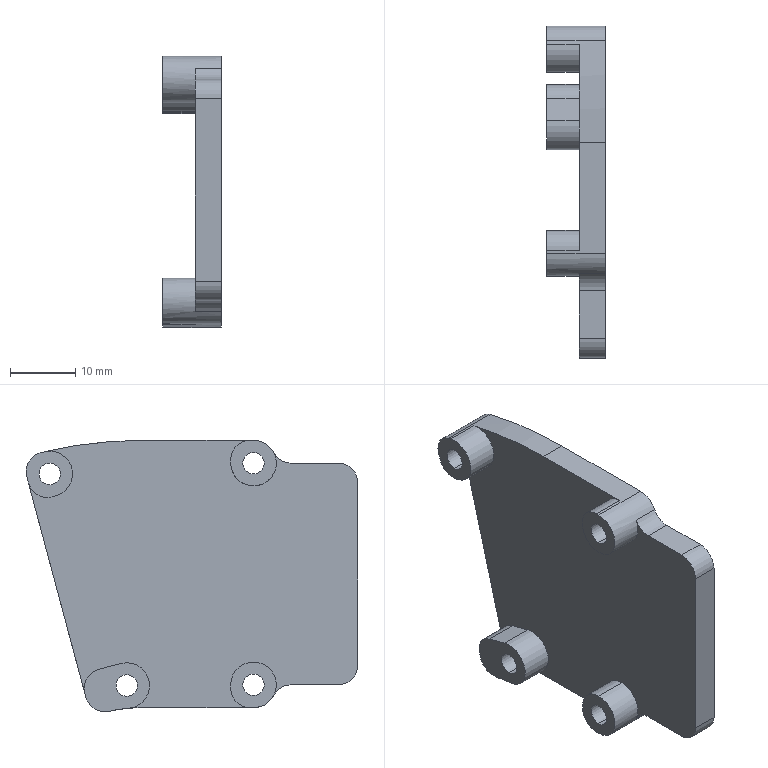Part | SolidWorks | features Extrusion 1, Fillet 1, ICE 1 | 1 solid | 42 faces | box 9 x 50.866 x 41.619 mm | volume 7798 mm3 | cylinder 26 | plane 16 | commonest cylinder face diameters 6 x11 3.3 x8 7 x5 49 x1 131 x1
STEP:
#1=CARTESIAN_POINT('',(-5.,31.604,11.728));
#2=VERTEX_POINT('',#1);
#3=CARTESIAN_POINT('',(-5.,30.827,11.83));
#4=VERTEX_POINT('',#3);
#5=CARTESIAN_POINT('',(-5.,31.604,14.728));
#6=DIRECTION('',(-1.,0.,0.));
#7=DIRECTION('',(0.,0.,1.));
#8=AXIS2_PLACEMENT_3D('',#5,#6,#7);
#9=CIRCLE('',#8,3.);
#10=EDGE_CURVE('',#2,#4,#9,.T.);
#11=ORIENTED_EDGE('',*,*,#10,.F.);
#12=CARTESIAN_POINT('',(0.,31.604,11.728));
#13=VERTEX_POINT('',#12);
#14=CARTESIAN_POINT('',(-5.,31.604,11.728));
#15=DIRECTION('',(1.,0.,0.));
#16=VECTOR('',#15,1000.);
#17=LINE('',#14,#16);
#18=EDGE_CURVE('',#2,#13,#17,.T.);
#19=ORIENTED_EDGE('',*,*,#18,.T.);
#20=CARTESIAN_POINT('',(0.,30.827,11.83));
#21=VERTEX_POINT('',#20);
#22=CARTESIAN_POINT('',(0.,31.604,14.728));
#23=DIRECTION('',(1.,0.,0.));
#24=DIRECTION('',(0.,0.,-1.));
#25=AXIS2_PLACEMENT_3D('',#22,#23,#24);
#26=CIRCLE('',#25,3.);
#27=EDGE_CURVE('',#21,#13,#26,.T.);
#28=ORIENTED_EDGE('',*,*,#27,.F.);
#29=CARTESIAN_POINT('',(-5.,30.827,11.83));
#30=DIRECTION('',(1.,0.,0.));
#31=VECTOR('',#30,1000.);
#32=LINE('',#29,#31);
#33=EDGE_CURVE('',#4,#21,#32,.T.);
#34=ORIENTED_EDGE('',*,*,#33,.F.);
#35=EDGE_LOOP('',(#11,#19,#28,#34));
#36=FACE_OUTER_BOUND('',#35,.T.);
#37=CARTESIAN_POINT('',(-5.,31.604,14.728));
#38=DIRECTION('',(1.,0.,0.));
#39=DIRECTION('',(0.,0.,-1.));
#40=AXIS2_PLACEMENT_3D('',#37,#38,#39);
#41=CYLINDRICAL_SURFACE('',#40,3.);
#42=ADVANCED_FACE('',(#36),#41,.T.);
#43=CARTESIAN_POINT('',(4.,19.44,-15.457));
#44=VERTEX_POINT('',#43);
#45=CARTESIAN_POINT('',(4.,19.44,-18.757));
#46=VERTEX_POINT('',#45);
#47=CARTESIAN_POINT('',(4.,19.44,-17.107));
#48=DIRECTION('',(1.,0.,0.));
#49=DIRECTION('',(0.,0.,-1.));
#50=AXIS2_PLACEMENT_3D('',#47,#48,#49);
#51=CIRCLE('',#50,1.65);
#52=EDGE_CURVE('',#44,#46,#51,.T.);
#53=ORIENTED_EDGE('',*,*,#52,.T.);
#54=CARTESIAN_POINT('',(-5.,19.44,-18.757));
#55=VERTEX_POINT('',#54);
#56=CARTESIAN_POINT('',(4.,19.44,-18.757));
#57=DIRECTION('',(-1.,0.,0.));
#58=VECTOR('',#57,1000.);
#59=LINE('',#56,#58);
#60=EDGE_CURVE('',#46,#55,#59,.T.);
#61=ORIENTED_EDGE('',*,*,#60,.T.);
#62=CARTESIAN_POINT('',(-5.,19.44,-15.457));
#63=VERTEX_POINT('',#62);
#64=CARTESIAN_POINT('',(-5.,19.44,-17.107));
#65=DIRECTION('',(-1.,0.,0.));
#66=DIRECTION('',(0.,0.,1.));
#67=AXIS2_PLACEMENT_3D('',#64,#65,#66);
#68=CIRCLE('',#67,1.65);
#69=EDGE_CURVE('',#55,#63,#68,.T.);
#70=ORIENTED_EDGE('',*,*,#69,.T.);
#71=CARTESIAN_POINT('',(4.,19.44,-15.457));
#72=DIRECTION('',(-1.,0.,0.));
#73=VECTOR('',#72,1000.);
#74=LINE('',#71,#73);
#75=EDGE_CURVE('',#44,#63,#74,.T.);
#76=ORIENTED_EDGE('',*,*,#75,.F.);
#77=EDGE_LOOP('',(#53,#61,#70,#76));
#78=FACE_OUTER_BOUND('',#77,.T.);
#79=CARTESIAN_POINT('',(4.,19.44,-17.107));
#80=DIRECTION('',(-1.,0.,0.));
#81=DIRECTION('',(0.,0.,1.));
#82=AXIS2_PLACEMENT_3D('',#79,#80,#81);
#83=CYLINDRICAL_SURFACE('',#82,1.65);
#84=ADVANCED_FACE('',(#78),#83,.F.);
#85=CARTESIAN_POINT('',(4.,31.25,16.99));
#86=VERTEX_POINT('',#85);
#87=CARTESIAN_POINT('',(4.,31.25,13.69));
#88=VERTEX_POINT('',#87);
#89=CARTESIAN_POINT('',(4.,31.25,15.34));
#90=DIRECTION('',(1.,0.,0.));
#91=DIRECTION('',(0.,0.,-1.));
#92=AXIS2_PLACEMENT_3D('',#89,#90,#91);
#93=CIRCLE('',#92,1.65);
#94=EDGE_CURVE('',#86,#88,#93,.T.);
#95=ORIENTED_EDGE('',*,*,#94,.T.);
#96=CARTESIAN_POINT('',(-5.,31.25,13.69));
#97=VERTEX_POINT('',#96);
#98=CARTESIAN_POINT('',(4.,31.25,13.69));
#99=DIRECTION('',(-1.,0.,0.));
#100=VECTOR('',#99,1000.);
#101=LINE('',#98,#100);
#102=EDGE_CURVE('',#88,#97,#101,.T.);
#103=ORIENTED_EDGE('',*,*,#102,.T.);
#104=CARTESIAN_POINT('',(-5.,31.25,16.99));
#105=VERTEX_POINT('',#104);
#106=CARTESIAN_POINT('',(-5.,31.25,15.34));
#107=DIRECTION('',(-1.,0.,0.));
#108=DIRECTION('',(0.,0.,1.));
#109=AXIS2_PLACEMENT_3D('',#106,#107,#108);
#110=CIRCLE('',#109,1.65);
#111=EDGE_CURVE('',#97,#105,#110,.T.);
#112=ORIENTED_EDGE('',*,*,#111,.T.);
#113=CARTESIAN_POINT('',(4.,31.25,16.99));
#114=DIRECTION('',(-1.,0.,0.));
#115=VECTOR('',#114,1000.);
#116=LINE('',#113,#115);
#117=EDGE_CURVE('',#86,#105,#116,.T.);
#118=ORIENTED_EDGE('',*,*,#117,.F.);
#119=EDGE_LOOP('',(#95,#103,#112,#118));
#120=FACE_OUTER_BOUND('',#119,.T.);
#121=CARTESIAN_POINT('',(4.,31.25,15.34));
#122=DIRECTION('',(-1.,0.,0.));
#123=DIRECTION('',(0.,0.,1.));
#124=AXIS2_PLACEMENT_3D('',#121,#122,#123);
#125=CYLINDRICAL_SURFACE('',#124,1.65);
#126=ADVANCED_FACE('',(#120),#125,.F.);
#127=CARTESIAN_POINT('',(4.,0.,-15.35));
#128=VERTEX_POINT('',#127);
#129=CARTESIAN_POINT('',(4.,0.,-18.65));
#130=VERTEX_POINT('',#129);
#131=CARTESIAN_POINT('',(4.,0.,-17.));
#132=DIRECTION('',(1.,0.,0.));
#133=DIRECTION('',(0.,0.,-1.));
#134=AXIS2_PLACEMENT_3D('',#131,#132,#133);
#135=CIRCLE('',#134,1.65);
#136=EDGE_CURVE('',#128,#130,#135,.T.);
#137=ORIENTED_EDGE('',*,*,#136,.T.);
#138=CARTESIAN_POINT('',(-5.,0.,-18.65));
#139=VERTEX_POINT('',#138);
#140=CARTESIAN_POINT('',(4.,0.,-18.65));
#141=DIRECTION('',(-1.,0.,0.));
#142=VECTOR('',#141,1000.);
#143=LINE('',#140,#142);
#144=EDGE_CURVE('',#130,#139,#143,.T.);
#145=ORIENTED_EDGE('',*,*,#144,.T.);
#146=CARTESIAN_POINT('',(-5.,0.,-15.35));
#147=VERTEX_POINT('',#146);
#148=CARTESIAN_POINT('',(-5.,0.,-17.));
#149=DIRECTION('',(-1.,0.,0.));
#150=DIRECTION('',(0.,0.,1.));
#151=AXIS2_PLACEMENT_3D('',#148,#149,#150);
#152=CIRCLE('',#151,1.65);
#153=EDGE_CURVE('',#139,#147,#152,.T.);
#154=ORIENTED_EDGE('',*,*,#153,.T.);
#155=CARTESIAN_POINT('',(4.,0.,-15.35));
#156=DIRECTION('',(-1.,0.,0.));
#157=VECTOR('',#156,1000.);
#158=LINE('',#155,#157);
#159=EDGE_CURVE('',#128,#147,#158,.T.);
#160=ORIENTED_EDGE('',*,*,#159,.F.);
#161=EDGE_LOOP('',(#137,#145,#154,#160));
#162=FACE_OUTER_BOUND('',#161,.T.);
#163=CARTESIAN_POINT('',(4.,0.,-17.));
#164=DIRECTION('',(-1.,0.,0.));
#165=DIRECTION('',(0.,0.,1.));
#166=AXIS2_PLACEMENT_3D('',#163,#164,#165);
#167=CYLINDRICAL_SURFACE('',#166,1.65);
#168=ADVANCED_FACE('',(#162),#167,.F.);
#169=CARTESIAN_POINT('',(4.,0.,18.65));
#170=VERTEX_POINT('',#169);
#171=CARTESIAN_POINT('',(4.,0.,15.35));
#172=VERTEX_POINT('',#171);
#173=CARTESIAN_POINT('',(4.,0.,17.));
#174=DIRECTION('',(1.,0.,0.));
#175=DIRECTION('',(0.,0.,-1.));
#176=AXIS2_PLACEMENT_3D('',#173,#174,#175);
#177=CIRCLE('',#176,1.65);
#178=EDGE_CURVE('',#170,#172,#177,.T.);
#179=ORIENTED_EDGE('',*,*,#178,.T.);
#180=CARTESIAN_POINT('',(-5.,0.,15.35));
#181=VERTEX_POINT('',#180);
#182=CARTESIAN_POINT('',(4.,0.,15.35));
#183=DIRECTION('',(-1.,0.,0.));
#184=VECTOR('',#183,1000.);
#185=LINE('',#182,#184);
#186=EDGE_CURVE('',#172,#181,#185,.T.);
#187=ORIENTED_EDGE('',*,*,#186,.T.);
#188=CARTESIAN_POINT('',(-5.,0.,18.65));
#189=VERTEX_POINT('',#188);
#190=CARTESIAN_POINT('',(-5.,0.,17.));
#191=DIRECTION('',(-1.,0.,0.));
#192=DIRECTION('',(0.,0.,1.));
#193=AXIS2_PLACEMENT_3D('',#190,#191,#192);
#194=CIRCLE('',#193,1.65);
#195=EDGE_CURVE('',#181,#189,#194,.T.);
#196=ORIENTED_EDGE('',*,*,#195,.T.);
#197=CARTESIAN_POINT('',(4.,0.,18.65));
#198=DIRECTION('',(-1.,0.,0.));
#199=VECTOR('',#198,1000.);
#200=LINE('',#197,#199);
#201=EDGE_CURVE('',#170,#189,#200,.T.);
#202=ORIENTED_EDGE('',*,*,#201,.F.);
#203=EDGE_LOOP('',(#179,#187,#196,#202));
#204=FACE_OUTER_BOUND('',#203,.T.);
#205=CARTESIAN_POINT('',(4.,0.,17.));
#206=DIRECTION('',(-1.,0.,0.));
#207=DIRECTION('',(0.,0.,1.));
#208=AXIS2_PLACEMENT_3D('',#205,#206,#207);
#209=CYLINDRICAL_SURFACE('',#208,1.65);
#210=ADVANCED_FACE('',(#204),#209,.F.);
#211=CARTESIAN_POINT('',(0.,-3.105,-18.615));
#212=VERTEX_POINT('',#211);
#213=CARTESIAN_POINT('',(0.,0.,-13.5));
#214=VERTEX_POINT('',#213);
#215=CARTESIAN_POINT('',(0.,0.,-17.));
#216=DIRECTION('',(-1.,0.,0.));
#217=DIRECTION('',(0.,0.,1.));
#218=AXIS2_PLACEMENT_3D('',#215,#216,#217);
#219=CIRCLE('',#218,3.5);
#220=EDGE_CURVE('',#212,#214,#219,.T.);
#221=ORIENTED_EDGE('',*,*,#220,.T.);
#222=CARTESIAN_POINT('',(-5.,0.,-13.5));
#223=VERTEX_POINT('',#222);
#224=CARTESIAN_POINT('',(4.,0.,-13.5));
#225=DIRECTION('',(-1.,0.,0.));
#226=VECTOR('',#225,1000.);
#227=LINE('',#224,#226);
#228=EDGE_CURVE('',#214,#223,#227,.T.);
#229=ORIENTED_EDGE('',*,*,#228,.T.);
#230=CARTESIAN_POINT('',(-5.,0.,-20.5));
#231=VERTEX_POINT('',#230);
#232=CARTESIAN_POINT('',(-5.,0.,-17.));
#233=DIRECTION('',(-1.,0.,0.));
#234=DIRECTION('',(0.,0.,1.));
#235=AXIS2_PLACEMENT_3D('',#232,#233,#234);
#236=CIRCLE('',#235,3.5);
#237=EDGE_CURVE('',#231,#223,#236,.T.);
#238=ORIENTED_EDGE('',*,*,#237,.F.);
#239=CARTESIAN_POINT('',(4.,0.,-20.5));
#240=VERTEX_POINT('',#239);
#241=CARTESIAN_POINT('',(4.,0.,-20.5));
#242=DIRECTION('',(-1.,0.,0.));
#243=VECTOR('',#242,1000.);
#244=LINE('',#241,#243);
#245=EDGE_CURVE('',#240,#231,#244,.T.);
#246=ORIENTED_EDGE('',*,*,#245,.F.);
#247=CARTESIAN_POINT('',(4.,-3.105,-18.615));
#248=VERTEX_POINT('',#247);
#249=CARTESIAN_POINT('',(4.,0.,-17.));
#250=DIRECTION('',(1.,0.,0.));
#251=DIRECTION('',(0.,0.,-1.));
#252=AXIS2_PLACEMENT_3D('',#249,#250,#251);
#253=CIRCLE('',#252,3.5);
#254=EDGE_CURVE('',#248,#240,#253,.T.);
#255=ORIENTED_EDGE('',*,*,#254,.F.);
#256=CARTESIAN_POINT('',(4.,-3.105,-18.615));
#257=DIRECTION('',(-1.,0.,0.));
#258=VECTOR('',#257,1000.);
#259=LINE('',#256,#258);
#260=EDGE_CURVE('',#248,#212,#259,.T.);
#261=ORIENTED_EDGE('',*,*,#260,.T.);
#262=EDGE_LOOP('',(#221,#229,#238,#246,#255,#261));
#263=FACE_OUTER_BOUND('',#262,.T.);
#264=CARTESIAN_POINT('',(4.,0.,-17.));
#265=DIRECTION('',(-1.,0.,0.));
#266=DIRECTION('',(0.,0.,1.));
#267=AXIS2_PLACEMENT_3D('',#264,#265,#266);
#268=CYLINDRICAL_SURFACE('',#267,3.5);
#269=ADVANCED_FACE('',(#263),#268,.T.);
#270=CARTESIAN_POINT('',(0.,-13.,-17.));
#271=VERTEX_POINT('',#270);
#272=CARTESIAN_POINT('',(0.,-5.766,-17.));
#273=VERTEX_POINT('',#272);
#274=CARTESIAN_POINT('',(0.,-16.,-17.));
#275=DIRECTION('',(0.,1.,0.));
#276=VECTOR('',#275,1000.);
#277=LINE('',#274,#276);
#278=EDGE_CURVE('',#271,#273,#277,.T.);
#279=ORIENTED_EDGE('',*,*,#278,.F.);
#280=CARTESIAN_POINT('',(0.,-16.,-14.));
#281=VERTEX_POINT('',#280);
#282=CARTESIAN_POINT('',(0.,-13.,-14.));
#283=DIRECTION('',(-1.,0.,0.));
#284=DIRECTION('',(0.,0.,-1.));
#285=AXIS2_PLACEMENT_3D('',#282,#283,#284);
#286=CIRCLE('',#285,3.);
#287=EDGE_CURVE('',#271,#281,#286,.T.);
#288=ORIENTED_EDGE('',*,*,#287,.T.);
#289=CARTESIAN_POINT('',(0.,-16.,14.));
#290=VERTEX_POINT('',#289);
#291=CARTESIAN_POINT('',(0.,-16.,17.));
#292=DIRECTION('',(0.,0.,-1.));
#293=VECTOR('',#292,1000.);
#294=LINE('',#291,#293);
#295=EDGE_CURVE('',#290,#281,#294,.T.);
#296=ORIENTED_EDGE('',*,*,#295,.F.);
#297=CARTESIAN_POINT('',(0.,-13.,17.));
#298=VERTEX_POINT('',#297);
#299=CARTESIAN_POINT('',(0.,-13.,14.));
#300=DIRECTION('',(-1.,0.,0.));
#301=DIRECTION('',(0.,0.,-1.));
#302=AXIS2_PLACEMENT_3D('',#299,#300,#301);
#303=CIRCLE('',#302,3.);
#304=EDGE_CURVE('',#290,#298,#303,.T.);
#305=ORIENTED_EDGE('',*,*,#304,.T.);
#306=CARTESIAN_POINT('',(0.,-5.766,17.));
#307=VERTEX_POINT('',#306);
#308=CARTESIAN_POINT('',(0.,-3.5,17.));
#309=DIRECTION('',(0.,-1.,0.));
#310=VECTOR('',#309,1000.);
#311=LINE('',#308,#310);
#312=EDGE_CURVE('',#307,#298,#311,.T.);
#313=ORIENTED_EDGE('',*,*,#312,.F.);
#314=CARTESIAN_POINT('',(0.,-3.105,18.615));
#315=VERTEX_POINT('',#314);
#316=CARTESIAN_POINT('',(0.,-5.766,20.));
#317=DIRECTION('',(1.,0.,0.));
#318=DIRECTION('',(0.,0.,-1.));
#319=AXIS2_PLACEMENT_3D('',#316,#317,#318);
#320=CIRCLE('',#319,3.);
#321=EDGE_CURVE('',#307,#315,#320,.T.);
#322=ORIENTED_EDGE('',*,*,#321,.T.);
#323=CARTESIAN_POINT('',(0.,3.5,17.));
#324=VERTEX_POINT('',#323);
#325=CARTESIAN_POINT('',(0.,0.,17.));
#326=DIRECTION('',(-1.,0.,0.));
#327=DIRECTION('',(0.,0.,1.));
#328=AXIS2_PLACEMENT_3D('',#325,#326,#327);
#329=CIRCLE('',#328,3.5);
#330=EDGE_CURVE('',#324,#315,#329,.T.);
#331=ORIENTED_EDGE('',*,*,#330,.F.);
#332=CARTESIAN_POINT('',(0.,3.5,17.5));
#333=VERTEX_POINT('',#332);
#334=CARTESIAN_POINT('',(0.,3.5,17.));
#335=DIRECTION('',(0.,0.,-1.));
#336=VECTOR('',#335,1000.);
#337=LINE('',#334,#336);
#338=EDGE_CURVE('',#333,#324,#337,.T.);
#339=ORIENTED_EDGE('',*,*,#338,.F.);
#340=CARTESIAN_POINT('',(0.,0.5,20.5));
#341=VERTEX_POINT('',#340);
#342=CARTESIAN_POINT('',(0.,0.5,17.5));
#343=DIRECTION('',(1.,0.,0.));
#344=DIRECTION('',(0.,0.,-1.));
#345=AXIS2_PLACEMENT_3D('',#342,#343,#344);
#346=CIRCLE('',#345,3.);
#347=EDGE_CURVE('',#333,#341,#346,.T.);
#348=ORIENTED_EDGE('',*,*,#347,.T.);
#349=CARTESIAN_POINT('',(0.,17.,20.5));
#350=VERTEX_POINT('',#349);
#351=CARTESIAN_POINT('',(0.,17.,20.5));
#352=DIRECTION('',(0.,-1.,0.));
#353=VECTOR('',#352,1000.);
#354=LINE('',#351,#353);
#355=EDGE_CURVE('',#350,#341,#354,.T.);
#356=ORIENTED_EDGE('',*,*,#355,.F.);
#357=CARTESIAN_POINT('',(0.,32.054,18.746));
#358=VERTEX_POINT('',#357);
#359=CARTESIAN_POINT('',(0.,17.,-45.));
#360=DIRECTION('',(1.,0.,0.));
#361=DIRECTION('',(0.,0.,-1.));
#362=AXIS2_PLACEMENT_3D('',#359,#360,#361);
#363=CIRCLE('',#362,65.5);
#364=EDGE_CURVE('',#358,#350,#363,.T.);
#365=ORIENTED_EDGE('',*,*,#364,.F.);
#366=CARTESIAN_POINT('',(0.,30.344,11.959));
#367=VERTEX_POINT('',#366);
#368=CARTESIAN_POINT('',(0.,31.25,15.34));
#369=DIRECTION('',(-1.,0.,0.));
#370=DIRECTION('',(0.,0.,1.));
#371=AXIS2_PLACEMENT_3D('',#368,#369,#370);
#372=CIRCLE('',#371,3.5);
#373=EDGE_CURVE('',#367,#358,#372,.T.);
#374=ORIENTED_EDGE('',*,*,#373,.F.);
#375=CARTESIAN_POINT('',(0.,33.725,11.054));
#376=DIRECTION('',(0.,-0.9659,0.2588));
#377=VECTOR('',#376,1000.);
#378=LINE('',#375,#377);
#379=EDGE_CURVE('',#21,#367,#378,.T.);
#380=ORIENTED_EDGE('',*,*,#379,.F.);
#381=ORIENTED_EDGE('',*,*,#27,.T.);
#382=CARTESIAN_POINT('',(0.,34.501,13.951));
#383=VERTEX_POINT('',#382);
#384=CARTESIAN_POINT('',(0.,31.604,14.728));
#385=DIRECTION('',(1.,0.,0.));
#386=DIRECTION('',(0.,0.,-1.));
#387=AXIS2_PLACEMENT_3D('',#384,#385,#386);
#388=CIRCLE('',#387,3.);
#389=EDGE_CURVE('',#13,#383,#388,.T.);
#390=ORIENTED_EDGE('',*,*,#389,.T.);
#391=CARTESIAN_POINT('',(0.,25.857,-18.308));
#392=VERTEX_POINT('',#391);
#393=CARTESIAN_POINT('',(0.,35.538,17.822));
#394=DIRECTION('',(0.,0.2588,0.9659));
#395=VECTOR('',#394,1000.);
#396=LINE('',#393,#395);
#397=EDGE_CURVE('',#392,#383,#396,.T.);
#398=ORIENTED_EDGE('',*,*,#397,.F.);
#399=CARTESIAN_POINT('',(0.,23.736,-14.634));
#400=VERTEX_POINT('',#399);
#401=CARTESIAN_POINT('',(0.,22.96,-17.532));
#402=DIRECTION('',(1.,0.,0.));
#403=DIRECTION('',(0.,0.,-1.));
#404=AXIS2_PLACEMENT_3D('',#401,#402,#403);
#405=CIRCLE('',#404,3.);
#406=EDGE_CURVE('',#392,#400,#405,.T.);
#407=ORIENTED_EDGE('',*,*,#406,.T.);
#408=CARTESIAN_POINT('',(0.,20.346,-13.726));
#409=VERTEX_POINT('',#408);
#410=CARTESIAN_POINT('',(0.,20.346,-13.726));
#411=DIRECTION('',(0.,0.9659,-0.2588));
#412=VECTOR('',#411,1000.);
#413=LINE('',#410,#412);
#414=EDGE_CURVE('',#409,#400,#413,.T.);
#415=ORIENTED_EDGE('',*,*,#414,.F.);
#416=CARTESIAN_POINT('',(0.,19.135,-20.593));
#417=VERTEX_POINT('',#416);
#418=CARTESIAN_POINT('',(0.,19.44,-17.107));
#419=DIRECTION('',(-1.,0.,0.));
#420=DIRECTION('',(0.,0.,1.));
#421=AXIS2_PLACEMENT_3D('',#418,#419,#420);
#422=CIRCLE('',#421,3.5);
#423=EDGE_CURVE('',#417,#409,#422,.T.);
#424=ORIENTED_EDGE('',*,*,#423,.F.);
#425=CARTESIAN_POINT('',(0.,17.,-20.5));
#426=VERTEX_POINT('',#425);
#427=CARTESIAN_POINT('',(0.,17.,-45.));
#428=DIRECTION('',(-1.,0.,0.));
#429=DIRECTION('',(0.,0.,-1.));
#430=AXIS2_PLACEMENT_3D('',#427,#428,#429);
#431=CIRCLE('',#430,24.5);
#432=EDGE_CURVE('',#426,#417,#431,.T.);
#433=ORIENTED_EDGE('',*,*,#432,.F.);
#434=CARTESIAN_POINT('',(0.,0.5,-20.5));
#435=VERTEX_POINT('',#434);
#436=CARTESIAN_POINT('',(0.,17.,-20.5));
#437=DIRECTION('',(0.,1.,0.));
#438=VECTOR('',#437,1000.);
#439=LINE('',#436,#438);
#440=EDGE_CURVE('',#435,#426,#439,.T.);
#441=ORIENTED_EDGE('',*,*,#440,.F.);
#442=CARTESIAN_POINT('',(0.,3.5,-17.5));
#443=VERTEX_POINT('',#442);
#444=CARTESIAN_POINT('',(0.,0.5,-17.5));
#445=DIRECTION('',(1.,0.,0.));
#446=DIRECTION('',(0.,0.,-1.));
#447=AXIS2_PLACEMENT_3D('',#444,#445,#446);
#448=CIRCLE('',#447,3.);
#449=EDGE_CURVE('',#435,#443,#448,.T.);
#450=ORIENTED_EDGE('',*,*,#449,.T.);
#451=CARTESIAN_POINT('',(0.,3.5,-17.));
#452=VERTEX_POINT('',#451);
#453=CARTESIAN_POINT('',(0.,3.5,-17.));
#454=DIRECTION('',(0.,0.,-1.));
#455=VECTOR('',#454,1000.);
#456=LINE('',#453,#455);
#457=EDGE_CURVE('',#452,#443,#456,.T.);
#458=ORIENTED_EDGE('',*,*,#457,.F.);
#459=CARTESIAN_POINT('',(0.,0.,-17.));
#460=DIRECTION('',(-1.,0.,0.));
#461=DIRECTION('',(0.,0.,1.));
#462=AXIS2_PLACEMENT_3D('',#459,#460,#461);
#463=CIRCLE('',#462,3.5);
#464=EDGE_CURVE('',#214,#452,#463,.T.);
#465=ORIENTED_EDGE('',*,*,#464,.F.);
#466=ORIENTED_EDGE('',*,*,#220,.F.);
#467=CARTESIAN_POINT('',(0.,-5.766,-20.));
#468=DIRECTION('',(1.,0.,0.));
#469=DIRECTION('',(0.,0.,-1.));
#470=AXIS2_PLACEMENT_3D('',#467,#468,#469);
#471=CIRCLE('',#470,3.);
#472=EDGE_CURVE('',#212,#273,#471,.T.);
#473=ORIENTED_EDGE('',*,*,#472,.T.);
#474=EDGE_LOOP('',(#279,#288,#296,#305,#313,#322,#331,#339,#348,#356,#365,#374,#380,#381,#390,#398,#407,#415,#424,#433,#441,#450,#458,#465,#466,#473));
#475=FACE_OUTER_BOUND('',#474,.T.);
#476=CARTESIAN_POINT('',(0.,17.,-45.));
#477=DIRECTION('',(1.,0.,0.));
#478=DIRECTION('',(0.,0.,-1.));
#479=AXIS2_PLACEMENT_3D('',#476,#477,#478);
#480=PLANE('',#479);
#481=ADVANCED_FACE('',(#475),#480,.F.);
#482=ORIENTED_EDGE('',*,*,#94,.F.);
#483=CARTESIAN_POINT('',(4.,31.25,15.34));
#484=DIRECTION('',(1.,0.,0.));
#485=DIRECTION('',(0.,0.,-1.));
#486=AXIS2_PLACEMENT_3D('',#483,#484,#485);
#487=CIRCLE('',#486,1.65);
#488=EDGE_CURVE('',#88,#86,#487,.T.);
#489=ORIENTED_EDGE('',*,*,#488,.F.);
#490=EDGE_LOOP('',(#482,#489));
#491=FACE_BOUND('',#490,.T.);
#492=ORIENTED_EDGE('',*,*,#178,.F.);
#493=CARTESIAN_POINT('',(4.,0.,17.));
#494=DIRECTION('',(1.,0.,0.));
#495=DIRECTION('',(0.,0.,-1.));
#496=AXIS2_PLACEMENT_3D('',#493,#494,#495);
#497=CIRCLE('',#496,1.65);
#498=EDGE_CURVE('',#172,#170,#497,.T.);
#499=ORIENTED_EDGE('',*,*,#498,.F.);
#500=EDGE_LOOP('',(#492,#499));
#501=FACE_BOUND('',#500,.T.);
#502=CARTESIAN_POINT('',(4.,-16.,14.));
#503=VERTEX_POINT('',#502);
#504=CARTESIAN_POINT('',(4.,-16.,-14.));
#505=VERTEX_POINT('',#504);
#506=CARTESIAN_POINT('',(4.,-16.,17.));
#507=DIRECTION('',(0.,0.,-1.));
#508=VECTOR('',#507,1000.);
#509=LINE('',#506,#508);
#510=EDGE_CURVE('',#503,#505,#509,.T.);
#511=ORIENTED_EDGE('',*,*,#510,.T.);
#512=CARTESIAN_POINT('',(4.,-13.,-17.));
#513=VERTEX_POINT('',#512);
#514=CARTESIAN_POINT('',(4.,-13.,-14.));
#515=DIRECTION('',(1.,0.,0.));
#516=DIRECTION('',(0.,0.,-1.));
#517=AXIS2_PLACEMENT_3D('',#514,#515,#516);
#518=CIRCLE('',#517,3.);
#519=EDGE_CURVE('',#505,#513,#518,.T.);
#520=ORIENTED_EDGE('',*,*,#519,.T.);
#521=CARTESIAN_POINT('',(4.,-5.766,-17.));
#522=VERTEX_POINT('',#521);
#523=CARTESIAN_POINT('',(4.,-16.,-17.));
#524=DIRECTION('',(0.,1.,0.));
#525=VECTOR('',#524,1000.);
#526=LINE('',#523,#525);
#527=EDGE_CURVE('',#513,#522,#526,.T.);
#528=ORIENTED_EDGE('',*,*,#527,.T.);
#529=CARTESIAN_POINT('',(4.,-5.766,-20.));
#530=DIRECTION('',(-1.,0.,0.));
#531=DIRECTION('',(0.,0.,-1.));
#532=AXIS2_PLACEMENT_3D('',#529,#530,#531);
#533=CIRCLE('',#532,3.);
#534=EDGE_CURVE('',#522,#248,#533,.T.);
#535=ORIENTED_EDGE('',*,*,#534,.T.);
#536=ORIENTED_EDGE('',*,*,#254,.T.);
#537=CARTESIAN_POINT('',(4.,17.,-20.5));
#538=VERTEX_POINT('',#537);
#539=CARTESIAN_POINT('',(4.,17.,-20.5));
#540=DIRECTION('',(0.,1.,0.));
#541=VECTOR('',#540,1000.);
#542=LINE('',#539,#541);
#543=EDGE_CURVE('',#240,#538,#542,.T.);
#544=ORIENTED_EDGE('',*,*,#543,.T.);
#545=CARTESIAN_POINT('',(4.,22.169,-21.052));
#546=VERTEX_POINT('',#545);
#547=CARTESIAN_POINT('',(4.,17.,-45.));
#548=DIRECTION('',(-1.,0.,0.));
#549=DIRECTION('',(0.,0.,-1.));
#550=AXIS2_PLACEMENT_3D('',#547,#548,#549);
#551=CIRCLE('',#550,24.5);
#552=EDGE_CURVE('',#538,#546,#551,.T.);
#553=ORIENTED_EDGE('',*,*,#552,.T.);
#554=CARTESIAN_POINT('',(4.,25.7,-18.896));
#555=VERTEX_POINT('',#554);
#556=CARTESIAN_POINT('',(4.,22.802,-18.119));
#557=DIRECTION('',(1.,0.,0.));
#558=DIRECTION('',(0.,0.,-1.));
#559=AXIS2_PLACEMENT_3D('',#556,#557,#558);
#560=CIRCLE('',#559,3.);
#561=EDGE_CURVE('',#546,#555,#560,.T.);
#562=ORIENTED_EDGE('',*,*,#561,.T.);
#563=CARTESIAN_POINT('',(4.,34.764,14.93));
#564=VERTEX_POINT('',#563);
#565=CARTESIAN_POINT('',(4.,35.538,17.822));
#566=DIRECTION('',(0.,0.2588,0.9659));
#567=VECTOR('',#566,1000.);
#568=LINE('',#565,#567);
#569=EDGE_CURVE('',#555,#564,#568,.T.);
#570=ORIENTED_EDGE('',*,*,#569,.T.);
#571=CARTESIAN_POINT('',(4.,32.579,18.62));
#572=VERTEX_POINT('',#571);
#573=CARTESIAN_POINT('',(4.,31.866,15.706));
#574=DIRECTION('',(1.,0.,0.));
#575=DIRECTION('',(0.,0.,-1.));
#576=AXIS2_PLACEMENT_3D('',#573,#574,#575);
#577=CIRCLE('',#576,3.);
#578=EDGE_CURVE('',#564,#572,#577,.T.);
#579=ORIENTED_EDGE('',*,*,#578,.T.);
#580=CARTESIAN_POINT('',(4.,17.,20.5));
#581=VERTEX_POINT('',#580);
#582=CARTESIAN_POINT('',(4.,17.,-45.));
#583=DIRECTION('',(1.,0.,0.));
#584=DIRECTION('',(0.,0.,-1.));
#585=AXIS2_PLACEMENT_3D('',#582,#583,#584);
#586=CIRCLE('',#585,65.5);
#587=EDGE_CURVE('',#572,#581,#586,.T.);
#588=ORIENTED_EDGE('',*,*,#587,.T.);
#589=CARTESIAN_POINT('',(4.,0.,20.5));
#590=VERTEX_POINT('',#589);
#591=CARTESIAN_POINT('',(4.,17.,20.5));
#592=DIRECTION('',(0.,-1.,0.));
#593=VECTOR('',#592,1000.);
#594=LINE('',#591,#593);
#595=EDGE_CURVE('',#581,#590,#594,.T.);
#596=ORIENTED_EDGE('',*,*,#595,.T.);
#597=CARTESIAN_POINT('',(4.,-3.105,18.615));
#598=VERTEX_POINT('',#597);
#599=CARTESIAN_POINT('',(4.,0.,17.));
#600=DIRECTION('',(1.,0.,0.));
#601=DIRECTION('',(0.,0.,-1.));
#602=AXIS2_PLACEMENT_3D('',#599,#600,#601);
#603=CIRCLE('',#602,3.5);
#604=EDGE_CURVE('',#590,#598,#603,.T.);
#605=ORIENTED_EDGE('',*,*,#604,.T.);
#606=CARTESIAN_POINT('',(4.,-5.766,17.));
#607=VERTEX_POINT('',#606);
#608=CARTESIAN_POINT('',(4.,-5.766,20.));
#609=DIRECTION('',(-1.,0.,0.));
#610=DIRECTION('',(0.,0.,-1.));
#611=AXIS2_PLACEMENT_3D('',#608,#609,#610);
#612=CIRCLE('',#611,3.);
#613=EDGE_CURVE('',#598,#607,#612,.T.);
#614=ORIENTED_EDGE('',*,*,#613,.T.);
#615=CARTESIAN_POINT('',(4.,-13.,17.));
#616=VERTEX_POINT('',#615);
#617=CARTESIAN_POINT('',(4.,-3.5,17.));
#618=DIRECTION('',(0.,-1.,0.));
#619=VECTOR('',#618,1000.);
#620=LINE('',#617,#619);
#621=EDGE_CURVE('',#607,#616,#620,.T.);
#622=ORIENTED_EDGE('',*,*,#621,.T.);
#623=CARTESIAN_POINT('',(4.,-13.,14.));
#624=DIRECTION('',(1.,0.,0.));
#625=DIRECTION('',(0.,0.,-1.));
#626=AXIS2_PLACEMENT_3D('',#623,#624,#625);
#627=CIRCLE('',#626,3.);
#628=EDGE_CURVE('',#616,#503,#627,.T.);
#629=ORIENTED_EDGE('',*,*,#628,.T.);
#630=EDGE_LOOP('',(#511,#520,#528,#535,#536,#544,#553,#562,#570,#579,#588,#596,#605,#614,#622,#629));
#631=FACE_OUTER_BOUND('',#630,.T.);
#632=ORIENTED_EDGE('',*,*,#136,.F.);
#633=CARTESIAN_POINT('',(4.,0.,-17.));
#634=DIRECTION('',(1.,0.,0.));
#635=DIRECTION('',(0.,0.,-1.));
#636=AXIS2_PLACEMENT_3D('',#633,#634,#635);
#637=CIRCLE('',#636,1.65);
#638=EDGE_CURVE('',#130,#128,#637,.T.);
#639=ORIENTED_EDGE('',*,*,#638,.F.);
#640=EDGE_LOOP('',(#632,#639));
#641=FACE_BOUND('',#640,.T.);
#642=ORIENTED_EDGE('',*,*,#52,.F.);
#643=CARTESIAN_POINT('',(4.,19.44,-17.107));
#644=DIRECTION('',(1.,0.,0.));
#645=DIRECTION('',(0.,0.,-1.));
#646=AXIS2_PLACEMENT_3D('',#643,#644,#645);
#647=CIRCLE('',#646,1.65);
#648=EDGE_CURVE('',#46,#44,#647,.T.);
#649=ORIENTED_EDGE('',*,*,#648,.F.);
#650=EDGE_LOOP('',(#642,#649));
#651=FACE_BOUND('',#650,.T.);
#652=CARTESIAN_POINT('',(4.,17.,-45.));
#653=DIRECTION('',(1.,0.,0.));
#654=DIRECTION('',(0.,0.,-1.));
#655=AXIS2_PLACEMENT_3D('',#652,#653,#654);
#656=PLANE('',#655);
#657=ADVANCED_FACE('',(#491,#501,#631,#641,#651),#656,.T.);
#658=ORIENTED_EDGE('',*,*,#587,.F.);
#659=CARTESIAN_POINT('',(-5.,32.579,18.62));
#660=VERTEX_POINT('',#659);
#661=CARTESIAN_POINT('',(4.,32.579,18.62));
#662=DIRECTION('',(-1.,0.,0.));
#663=VECTOR('',#662,1000.);
#664=LINE('',#661,#663);
#665=EDGE_CURVE('',#572,#660,#664,.T.);
#666=ORIENTED_EDGE('',*,*,#665,.T.);
#667=CARTESIAN_POINT('',(-5.,32.054,18.746));
#668=VERTEX_POINT('',#667);
#669=CARTESIAN_POINT('',(-5.,17.,-45.));
#670=DIRECTION('',(-1.,0.,0.));
#671=DIRECTION('',(0.,0.,1.));
#672=AXIS2_PLACEMENT_3D('',#669,#670,#671);
#673=CIRCLE('',#672,65.5);
#674=EDGE_CURVE('',#668,#660,#673,.T.);
#675=ORIENTED_EDGE('',*,*,#674,.F.);
#676=CARTESIAN_POINT('',(-5.,32.054,18.746));
#677=DIRECTION('',(1.,0.,0.));
#678=VECTOR('',#677,1000.);
#679=LINE('',#676,#678);
#680=EDGE_CURVE('',#668,#358,#679,.T.);
#681=ORIENTED_EDGE('',*,*,#680,.T.);
#682=ORIENTED_EDGE('',*,*,#364,.T.);
#683=CARTESIAN_POINT('',(4.,17.,20.5));
#684=DIRECTION('',(-1.,0.,0.));
#685=VECTOR('',#684,1000.);
#686=LINE('',#683,#685);
#687=EDGE_CURVE('',#581,#350,#686,.T.);
#688=ORIENTED_EDGE('',*,*,#687,.F.);
#689=EDGE_LOOP('',(#658,#666,#675,#681,#682,#688));
#690=FACE_OUTER_BOUND('',#689,.T.);
#691=CARTESIAN_POINT('',(4.,17.,-45.));
#692=DIRECTION('',(-1.,0.,0.));
#693=DIRECTION('',(0.,0.,1.));
#694=AXIS2_PLACEMENT_3D('',#691,#692,#693);
#695=CYLINDRICAL_SURFACE('',#694,65.5);
#696=ADVANCED_FACE('',(#690),#695,.T.);
#697=ORIENTED_EDGE('',*,*,#355,.T.);
#698=CARTESIAN_POINT('',(-5.,0.5,20.5));
#699=VERTEX_POINT('',#698);
#700=CARTESIAN_POINT('',(4.,0.5,20.5));
#701=DIRECTION('',(-1.,0.,0.));
#702=VECTOR('',#701,1000.);
#703=LINE('',#700,#702);
#704=EDGE_CURVE('',#341,#699,#703,.T.);
#705=ORIENTED_EDGE('',*,*,#704,.T.);
#706=CARTESIAN_POINT('',(-5.,0.,20.5));
#707=VERTEX_POINT('',#706);
#708=CARTESIAN_POINT('',(-5.,3.5,20.5));
#709=DIRECTION('',(0.,1.,0.));
#710=VECTOR('',#709,1000.);
#711=LINE('',#708,#710);
#712=EDGE_CURVE('',#707,#699,#711,.T.);
#713=ORIENTED_EDGE('',*,*,#712,.F.);
#714=CARTESIAN_POINT('',(4.,0.,20.5));
#715=DIRECTION('',(-1.,0.,0.));
#716=VECTOR('',#715,1000.);
#717=LINE('',#714,#716);
#718=EDGE_CURVE('',#590,#707,#717,.T.);
#719=ORIENTED_EDGE('',*,*,#718,.F.);
#720=ORIENTED_EDGE('',*,*,#595,.F.);
#721=ORIENTED_EDGE('',*,*,#687,.T.);
#722=EDGE_LOOP('',(#697,#705,#713,#719,#720,#721));
#723=FACE_OUTER_BOUND('',#722,.T.);
#724=CARTESIAN_POINT('',(4.,17.,20.5));
#725=DIRECTION('',(0.,0.,-1.));
#726=DIRECTION('',(0.,1.,0.));
#727=AXIS2_PLACEMENT_3D('',#724,#725,#726);
#728=PLANE('',#727);
#729=ADVANCED_FACE('',(#723),#728,.F.);
#730=ORIENTED_EDGE('',*,*,#330,.T.);
#731=CARTESIAN_POINT('',(4.,-3.105,18.615));
#732=DIRECTION('',(1.,0.,0.));
#733=VECTOR('',#732,1000.);
#734=LINE('',#731,#733);
#735=EDGE_CURVE('',#315,#598,#734,.T.);
#736=ORIENTED_EDGE('',*,*,#735,.T.);
#737=ORIENTED_EDGE('',*,*,#604,.F.);
#738=ORIENTED_EDGE('',*,*,#718,.T.);
#739=CARTESIAN_POINT('',(-5.,3.5,17.));
#740=VERTEX_POINT('',#739);
#741=CARTESIAN_POINT('',(-5.,0.,17.));
#742=DIRECTION('',(-1.,0.,0.));
#743=DIRECTION('',(0.,0.,1.));
#744=AXIS2_PLACEMENT_3D('',#741,#742,#743);
#745=CIRCLE('',#744,3.5);
#746=EDGE_CURVE('',#740,#707,#745,.T.);
#747=ORIENTED_EDGE('',*,*,#746,.F.);
#748=CARTESIAN_POINT('',(-5.,3.5,17.));
#749=DIRECTION('',(1.,0.,0.));
#750=VECTOR('',#749,1000.);
#751=LINE('',#748,#750);
#752=EDGE_CURVE('',#740,#324,#751,.T.);
#753=ORIENTED_EDGE('',*,*,#752,.T.);
#754=EDGE_LOOP('',(#730,#736,#737,#738,#747,#753));
#755=FACE_OUTER_BOUND('',#754,.T.);
#756=CARTESIAN_POINT('',(4.,0.,17.));
#757=DIRECTION('',(-1.,0.,0.));
#758=DIRECTION('',(0.,0.,1.));
#759=AXIS2_PLACEMENT_3D('',#756,#757,#758);
#760=CYLINDRICAL_SURFACE('',#759,3.5);
#761=ADVANCED_FACE('',(#755),#760,.T.);
#762=ORIENTED_EDGE('',*,*,#312,.T.);
#763=CARTESIAN_POINT('',(4.,-13.,17.));
#764=DIRECTION('',(1.,0.,0.));
#765=VECTOR('',#764,1000.);
#766=LINE('',#763,#765);
#767=EDGE_CURVE('',#298,#616,#766,.T.);
#768=ORIENTED_EDGE('',*,*,#767,.T.);
#769=ORIENTED_EDGE('',*,*,#621,.F.);
#770=CARTESIAN_POINT('',(0.,-5.766,17.));
#771=DIRECTION('',(-1.,0.,0.));
#772=VECTOR('',#771,1000.);
#773=LINE('',#770,#772);
#774=EDGE_CURVE('',#607,#307,#773,.T.);
#775=ORIENTED_EDGE('',*,*,#774,.T.);
#776=EDGE_LOOP('',(#762,#768,#769,#775));
#777=FACE_OUTER_BOUND('',#776,.T.);
#778=CARTESIAN_POINT('',(4.,-3.5,17.));
#779=DIRECTION('',(0.,0.,-1.));
#780=DIRECTION('',(-1.,0.,0.));
#781=AXIS2_PLACEMENT_3D('',#778,#779,#780);
#782=PLANE('',#781);
#783=ADVANCED_FACE('',(#777),#782,.F.);
#784=ORIENTED_EDGE('',*,*,#295,.T.);
#785=CARTESIAN_POINT('',(4.,-16.,-14.));
#786=DIRECTION('',(1.,0.,0.));
#787=VECTOR('',#786,1000.);
#788=LINE('',#785,#787);
#789=EDGE_CURVE('',#281,#505,#788,.T.);
#790=ORIENTED_EDGE('',*,*,#789,.T.);
#791=ORIENTED_EDGE('',*,*,#510,.F.);
#792=CARTESIAN_POINT('',(4.,-16.,14.));
#793=DIRECTION('',(-1.,0.,0.));
#794=VECTOR('',#793,1000.);
#795=LINE('',#792,#794);
#796=EDGE_CURVE('',#503,#290,#795,.T.);
#797=ORIENTED_EDGE('',*,*,#796,.T.);
#798=EDGE_LOOP('',(#784,#790,#791,#797));
#799=FACE_OUTER_BOUND('',#798,.T.);
#800=CARTESIAN_POINT('',(4.,-16.,17.));
#801=DIRECTION('',(0.,1.,0.));
#802=DIRECTION('',(0.,0.,1.));
#803=AXIS2_PLACEMENT_3D('',#800,#801,#802);
#804=PLANE('',#803);
#805=ADVANCED_FACE('',(#799),#804,.F.);
#806=ORIENTED_EDGE('',*,*,#278,.T.);
#807=CARTESIAN_POINT('',(4.,-5.766,-17.));
#808=DIRECTION('',(1.,0.,0.));
#809=VECTOR('',#808,1000.);
#810=LINE('',#807,#809);
#811=EDGE_CURVE('',#273,#522,#810,.T.);
#812=ORIENTED_EDGE('',*,*,#811,.T.);
#813=ORIENTED_EDGE('',*,*,#527,.F.);
#814=CARTESIAN_POINT('',(4.,-13.,-17.));
#815=DIRECTION('',(-1.,0.,0.));
#816=VECTOR('',#815,1000.);
#817=LINE('',#814,#816);
#818=EDGE_CURVE('',#513,#271,#817,.T.);
#819=ORIENTED_EDGE('',*,*,#818,.T.);
#820=EDGE_LOOP('',(#806,#812,#813,#819));
#821=FACE_OUTER_BOUND('',#820,.T.);
#822=CARTESIAN_POINT('',(4.,-16.,-17.));
#823=DIRECTION('',(0.,0.,1.));
#824=DIRECTION('',(1.,0.,0.));
#825=AXIS2_PLACEMENT_3D('',#822,#823,#824);
#826=PLANE('',#825);
#827=ADVANCED_FACE('',(#821),#826,.F.);
#828=ORIENTED_EDGE('',*,*,#228,.F.);
#829=ORIENTED_EDGE('',*,*,#464,.T.);
#830=CARTESIAN_POINT('',(-5.,3.5,-17.));
#831=VERTEX_POINT('',#830);
#832=CARTESIAN_POINT('',(-5.,3.5,-17.));
#833=DIRECTION('',(1.,0.,0.));
#834=VECTOR('',#833,1000.);
#835=LINE('',#832,#834);
#836=EDGE_CURVE('',#831,#452,#835,.T.);
#837=ORIENTED_EDGE('',*,*,#836,.F.);
#838=CARTESIAN_POINT('',(-5.,0.,-17.));
#839=DIRECTION('',(-1.,0.,0.));
#840=DIRECTION('',(0.,0.,1.));
#841=AXIS2_PLACEMENT_3D('',#838,#839,#840);
#842=CIRCLE('',#841,3.5);
#843=EDGE_CURVE('',#223,#831,#842,.T.);
#844=ORIENTED_EDGE('',*,*,#843,.F.);
#845=EDGE_LOOP('',(#828,#829,#837,#844));
#846=FACE_OUTER_BOUND('',#845,.T.);
#847=CARTESIAN_POINT('',(4.,0.,-17.));
#848=DIRECTION('',(-1.,0.,0.));
#849=DIRECTION('',(0.,0.,1.));
#850=AXIS2_PLACEMENT_3D('',#847,#848,#849);
#851=CYLINDRICAL_SURFACE('',#850,3.5);
#852=ADVANCED_FACE('',(#846),#851,.T.);
#853=CARTESIAN_POINT('',(-5.,0.5,-20.5));
#854=VERTEX_POINT('',#853);
#855=CARTESIAN_POINT('',(-5.,0.,-20.5));
#856=DIRECTION('',(0.,-1.,0.));
#857=VECTOR('',#856,1000.);
#858=LINE('',#855,#857);
#859=EDGE_CURVE('',#854,#231,#858,.T.);
#860=ORIENTED_EDGE('',*,*,#859,.F.);
#861=CARTESIAN_POINT('',(4.,0.5,-20.5));
#862=DIRECTION('',(1.,0.,0.));
#863=VECTOR('',#862,1000.);
#864=LINE('',#861,#863);
#865=EDGE_CURVE('',#854,#435,#864,.T.);
#866=ORIENTED_EDGE('',*,*,#865,.T.);
#867=ORIENTED_EDGE('',*,*,#440,.T.);
#868=CARTESIAN_POINT('',(4.,17.,-20.5));
#869=DIRECTION('',(-1.,0.,0.));
#870=VECTOR('',#869,1000.);
#871=LINE('',#868,#870);
#872=EDGE_CURVE('',#538,#426,#871,.T.);
#873=ORIENTED_EDGE('',*,*,#872,.F.);
#874=ORIENTED_EDGE('',*,*,#543,.F.);
#875=ORIENTED_EDGE('',*,*,#245,.T.);
#876=EDGE_LOOP('',(#860,#866,#867,#873,#874,#875));
#877=FACE_OUTER_BOUND('',#876,.T.);
#878=CARTESIAN_POINT('',(4.,17.,-20.5));
#879=DIRECTION('',(0.,0.,1.));
#880=DIRECTION('',(0.,-1.,0.));
#881=AXIS2_PLACEMENT_3D('',#878,#879,#880);
#882=PLANE('',#881);
#883=ADVANCED_FACE('',(#877),#882,.F.);
#884=CARTESIAN_POINT('',(-5.,22.169,-21.052));
#885=VERTEX_POINT('',#884);
#886=CARTESIAN_POINT('',(-5.,19.135,-20.593));
#887=VERTEX_POINT('',#886);
#888=CARTESIAN_POINT('',(-5.,17.,-45.));
#889=DIRECTION('',(1.,0.,0.));
#890=DIRECTION('',(0.,0.,1.));
#891=AXIS2_PLACEMENT_3D('',#888,#889,#890);
#892=CIRCLE('',#891,24.5);
#893=EDGE_CURVE('',#885,#887,#892,.T.);
#894=ORIENTED_EDGE('',*,*,#893,.F.);
#895=CARTESIAN_POINT('',(4.,22.169,-21.052));
#896=DIRECTION('',(1.,0.,0.));
#897=VECTOR('',#896,1000.);
#898=LINE('',#895,#897);
#899=EDGE_CURVE('',#885,#546,#898,.T.);
#900=ORIENTED_EDGE('',*,*,#899,.T.);
#901=ORIENTED_EDGE('',*,*,#552,.F.);
#902=ORIENTED_EDGE('',*,*,#872,.T.);
#903=ORIENTED_EDGE('',*,*,#432,.T.);
#904=CARTESIAN_POINT('',(-5.,19.135,-20.593));
#905=DIRECTION('',(1.,0.,0.));
#906=VECTOR('',#905,1000.);
#907=LINE('',#904,#906);
#908=EDGE_CURVE('',#887,#417,#907,.T.);
#909=ORIENTED_EDGE('',*,*,#908,.F.);
#910=EDGE_LOOP('',(#894,#900,#901,#902,#903,#909));
#911=FACE_OUTER_BOUND('',#910,.T.);
#912=CARTESIAN_POINT('',(4.,17.,-45.));
#913=DIRECTION('',(-1.,0.,0.));
#914=DIRECTION('',(0.,0.,1.));
#915=AXIS2_PLACEMENT_3D('',#912,#913,#914);
#916=CYLINDRICAL_SURFACE('',#915,24.5);
#917=ADVANCED_FACE('',(#911),#916,.F.);
#918=CARTESIAN_POINT('',(-5.,25.857,-18.308));
#919=VERTEX_POINT('',#918);
#920=CARTESIAN_POINT('',(-5.,25.7,-18.896));
#921=VERTEX_POINT('',#920);
#922=CARTESIAN_POINT('',(-5.,24.918,-21.815));
#923=DIRECTION('',(0.,-0.2588,-0.9659));
#924=VECTOR('',#923,1000.);
#925=LINE('',#922,#924);
#926=EDGE_CURVE('',#919,#921,#925,.T.);
#927=ORIENTED_EDGE('',*,*,#926,.F.);
#928=CARTESIAN_POINT('',(4.,25.857,-18.308));
#929=DIRECTION('',(1.,0.,0.));
#930=VECTOR('',#929,1000.);
#931=LINE('',#928,#930);
#932=EDGE_CURVE('',#919,#392,#931,.T.);
#933=ORIENTED_EDGE('',*,*,#932,.T.);
#934=ORIENTED_EDGE('',*,*,#397,.T.);
#935=CARTESIAN_POINT('',(-5.,34.501,13.951));
#936=VERTEX_POINT('',#935);
#937=CARTESIAN_POINT('',(4.,34.501,13.951));
#938=DIRECTION('',(-1.,0.,0.));
#939=VECTOR('',#938,1000.);
#940=LINE('',#937,#939);
#941=EDGE_CURVE('',#383,#936,#940,.T.);
#942=ORIENTED_EDGE('',*,*,#941,.T.);
#943=CARTESIAN_POINT('',(-5.,34.764,14.93));
#944=VERTEX_POINT('',#943);
#945=CARTESIAN_POINT('',(-5.,33.725,11.054));
#946=DIRECTION('',(0.,-0.2588,-0.9659));
#947=VECTOR('',#946,1000.);
#948=LINE('',#945,#947);
#949=EDGE_CURVE('',#944,#936,#948,.T.);
#950=ORIENTED_EDGE('',*,*,#949,.F.);
#951=CARTESIAN_POINT('',(4.,34.764,14.93));
#952=DIRECTION('',(1.,0.,0.));
#953=VECTOR('',#952,1000.);
#954=LINE('',#951,#953);
#955=EDGE_CURVE('',#944,#564,#954,.T.);
#956=ORIENTED_EDGE('',*,*,#955,.T.);
#957=ORIENTED_EDGE('',*,*,#569,.F.);
#958=CARTESIAN_POINT('',(4.,25.7,-18.896));
#959=DIRECTION('',(-1.,0.,0.));
#960=VECTOR('',#959,1000.);
#961=LINE('',#958,#960);
#962=EDGE_CURVE('',#555,#921,#961,.T.);
#963=ORIENTED_EDGE('',*,*,#962,.T.);
#964=EDGE_LOOP('',(#927,#933,#934,#942,#950,#956,#957,#963));
#965=FACE_OUTER_BOUND('',#964,.T.);
#966=CARTESIAN_POINT('',(4.,35.538,17.822));
#967=DIRECTION('',(0.,-0.9659,0.2588));
#968=DIRECTION('',(0.,-0.2588,-0.9659));
#969=AXIS2_PLACEMENT_3D('',#966,#967,#968);
#970=PLANE('',#969);
#971=ADVANCED_FACE('',(#965),#970,.F.);
#972=ORIENTED_EDGE('',*,*,#186,.F.);
#973=ORIENTED_EDGE('',*,*,#498,.T.);
#974=ORIENTED_EDGE('',*,*,#201,.T.);
#975=CARTESIAN_POINT('',(-5.,0.,17.));
#976=DIRECTION('',(-1.,0.,0.));
#977=DIRECTION('',(0.,0.,1.));
#978=AXIS2_PLACEMENT_3D('',#975,#976,#977);
#979=CIRCLE('',#978,1.65);
#980=EDGE_CURVE('',#189,#181,#979,.T.);
#981=ORIENTED_EDGE('',*,*,#980,.T.);
#982=EDGE_LOOP('',(#972,#973,#974,#981));
#983=FACE_OUTER_BOUND('',#982,.T.);
#984=CARTESIAN_POINT('',(4.,0.,17.));
#985=DIRECTION('',(-1.,0.,0.));
#986=DIRECTION('',(0.,0.,1.));
#987=AXIS2_PLACEMENT_3D('',#984,#985,#986);
#988=CYLINDRICAL_SURFACE('',#987,1.65);
#989=ADVANCED_FACE('',(#983),#988,.F.);
#990=ORIENTED_EDGE('',*,*,#144,.F.);
#991=ORIENTED_EDGE('',*,*,#638,.T.);
#992=ORIENTED_EDGE('',*,*,#159,.T.);
#993=CARTESIAN_POINT('',(-5.,0.,-17.));
#994=DIRECTION('',(-1.,0.,0.));
#995=DIRECTION('',(0.,0.,1.));
#996=AXIS2_PLACEMENT_3D('',#993,#994,#995);
#997=CIRCLE('',#996,1.65);
#998=EDGE_CURVE('',#147,#139,#997,.T.);
#999=ORIENTED_EDGE('',*,*,#998,.T.);
#1000=EDGE_LOOP('',(#990,#991,#992,#999));
#1001=FACE_OUTER_BOUND('',#1000,.T.);
#1002=CARTESIAN_POINT('',(4.,0.,-17.));
#1003=DIRECTION('',(-1.,0.,0.));
#1004=DIRECTION('',(0.,0.,1.));
#1005=AXIS2_PLACEMENT_3D('',#1002,#1003,#1004);
#1006=CYLINDRICAL_SURFACE('',#1005,1.65);
#1007=ADVANCED_FACE('',(#1001),#1006,.F.);
#1008=ORIENTED_EDGE('',*,*,#102,.F.);
#1009=ORIENTED_EDGE('',*,*,#488,.T.);
#1010=ORIENTED_EDGE('',*,*,#117,.T.);
#1011=CARTESIAN_POINT('',(-5.,31.25,15.34));
#1012=DIRECTION('',(-1.,0.,0.));
#1013=DIRECTION('',(0.,0.,1.));
#1014=AXIS2_PLACEMENT_3D('',#1011,#1012,#1013);
#1015=CIRCLE('',#1014,1.65);
#1016=EDGE_CURVE('',#105,#97,#1015,.T.);
#1017=ORIENTED_EDGE('',*,*,#1016,.T.);
#1018=EDGE_LOOP('',(#1008,#1009,#1010,#1017));
#1019=FACE_OUTER_BOUND('',#1018,.T.);
#1020=CARTESIAN_POINT('',(4.,31.25,15.34));
#1021=DIRECTION('',(-1.,0.,0.));
#1022=DIRECTION('',(0.,0.,1.));
#1023=AXIS2_PLACEMENT_3D('',#1020,#1021,#1022);
#1024=CYLINDRICAL_SURFACE('',#1023,1.65);
#1025=ADVANCED_FACE('',(#1019),#1024,.F.);
#1026=ORIENTED_EDGE('',*,*,#60,.F.);
#1027=ORIENTED_EDGE('',*,*,#648,.T.);
#1028=ORIENTED_EDGE('',*,*,#75,.T.);
#1029=CARTESIAN_POINT('',(-5.,19.44,-17.107));
#1030=DIRECTION('',(-1.,0.,0.));
#1031=DIRECTION('',(0.,0.,1.));
#1032=AXIS2_PLACEMENT_3D('',#1029,#1030,#1031);
#1033=CIRCLE('',#1032,1.65);
#1034=EDGE_CURVE('',#63,#55,#1033,.T.);
#1035=ORIENTED_EDGE('',*,*,#1034,.T.);
#1036=EDGE_LOOP('',(#1026,#1027,#1028,#1035));
#1037=FACE_OUTER_BOUND('',#1036,.T.);
#1038=CARTESIAN_POINT('',(4.,19.44,-17.107));
#1039=DIRECTION('',(-1.,0.,0.));
#1040=DIRECTION('',(0.,0.,1.));
#1041=AXIS2_PLACEMENT_3D('',#1038,#1039,#1040);
#1042=CYLINDRICAL_SURFACE('',#1041,1.65);
#1043=ADVANCED_FACE('',(#1037),#1042,.F.);
#1044=ORIENTED_EDGE('',*,*,#949,.T.);
#1045=CARTESIAN_POINT('',(-5.,31.604,14.728));
#1046=DIRECTION('',(-1.,0.,0.));
#1047=DIRECTION('',(0.,0.,1.));
#1048=AXIS2_PLACEMENT_3D('',#1045,#1046,#1047);
#1049=CIRCLE('',#1048,3.);
#1050=EDGE_CURVE('',#936,#2,#1049,.T.);
#1051=ORIENTED_EDGE('',*,*,#1050,.T.);
#1052=ORIENTED_EDGE('',*,*,#10,.T.);
#1053=CARTESIAN_POINT('',(-5.,30.344,11.959));
#1054=VERTEX_POINT('',#1053);
#1055=CARTESIAN_POINT('',(-5.,33.725,11.054));
#1056=DIRECTION('',(0.,-0.9659,0.2588));
#1057=VECTOR('',#1056,1000.);
#1058=LINE('',#1055,#1057);
#1059=EDGE_CURVE('',#4,#1054,#1058,.T.);
#1060=ORIENTED_EDGE('',*,*,#1059,.T.);
#1061=CARTESIAN_POINT('',(-5.,31.25,15.34));
#1062=DIRECTION('',(-1.,0.,0.));
#1063=DIRECTION('',(0.,0.,1.));
#1064=AXIS2_PLACEMENT_3D('',#1061,#1062,#1063);
#1065=CIRCLE('',#1064,3.5);
#1066=EDGE_CURVE('',#1054,#668,#1065,.T.);
#1067=ORIENTED_EDGE('',*,*,#1066,.T.);
#1068=ORIENTED_EDGE('',*,*,#674,.T.);
#1069=CARTESIAN_POINT('',(-5.,31.866,15.706));
#1070=DIRECTION('',(-1.,0.,0.));
#1071=DIRECTION('',(0.,0.,1.));
#1072=AXIS2_PLACEMENT_3D('',#1069,#1070,#1071);
#1073=CIRCLE('',#1072,3.);
#1074=EDGE_CURVE('',#660,#944,#1073,.T.);
#1075=ORIENTED_EDGE('',*,*,#1074,.T.);
#1076=EDGE_LOOP('',(#1044,#1051,#1052,#1060,#1067,#1068,#1075));
#1077=FACE_OUTER_BOUND('',#1076,.T.);
#1078=ORIENTED_EDGE('',*,*,#1016,.F.);
#1079=ORIENTED_EDGE('',*,*,#111,.F.);
#1080=EDGE_LOOP('',(#1078,#1079));
#1081=FACE_BOUND('',#1080,.T.);
#1082=CARTESIAN_POINT('',(-5.,31.25,15.34));
#1083=DIRECTION('',(-1.,0.,0.));
#1084=DIRECTION('',(0.,0.,1.));
#1085=AXIS2_PLACEMENT_3D('',#1082,#1083,#1084);
#1086=PLANE('',#1085);
#1087=ADVANCED_FACE('',(#1077,#1081),#1086,.T.);
#1088=ORIENTED_EDGE('',*,*,#1059,.F.);
#1089=ORIENTED_EDGE('',*,*,#33,.T.);
#1090=ORIENTED_EDGE('',*,*,#379,.T.);
#1091=CARTESIAN_POINT('',(-5.,30.344,11.959));
#1092=DIRECTION('',(1.,0.,0.));
#1093=VECTOR('',#1092,1000.);
#1094=LINE('',#1091,#1093);
#1095=EDGE_CURVE('',#1054,#367,#1094,.T.);
#1096=ORIENTED_EDGE('',*,*,#1095,.F.);
#1097=EDGE_LOOP('',(#1088,#1089,#1090,#1096));
#1098=FACE_OUTER_BOUND('',#1097,.T.);
#1099=CARTESIAN_POINT('',(-5.,33.725,11.054));
#1100=DIRECTION('',(0.,0.2588,0.9659));
#1101=DIRECTION('',(0.,-0.9659,0.2588));
#1102=AXIS2_PLACEMENT_3D('',#1099,#1100,#1101);
#1103=PLANE('',#1102);
#1104=ADVANCED_FACE('',(#1098),#1103,.F.);
#1105=ORIENTED_EDGE('',*,*,#373,.T.);
#1106=ORIENTED_EDGE('',*,*,#680,.F.);
#1107=ORIENTED_EDGE('',*,*,#1066,.F.);
#1108=ORIENTED_EDGE('',*,*,#1095,.T.);
#1109=EDGE_LOOP('',(#1105,#1106,#1107,#1108));
#1110=FACE_OUTER_BOUND('',#1109,.T.);
#1111=CARTESIAN_POINT('',(-5.,31.25,15.34));
#1112=DIRECTION('',(1.,0.,0.));
#1113=DIRECTION('',(0.,0.,-1.));
#1114=AXIS2_PLACEMENT_3D('',#1111,#1112,#1113);
#1115=CYLINDRICAL_SURFACE('',#1114,3.5);
#1116=ADVANCED_FACE('',(#1110),#1115,.T.);
#1117=CARTESIAN_POINT('',(-5.,3.5,-17.5));
#1118=VERTEX_POINT('',#1117);
#1119=CARTESIAN_POINT('',(-5.,3.5,-17.));
#1120=DIRECTION('',(0.,0.,-1.));
#1121=VECTOR('',#1120,1000.);
#1122=LINE('',#1119,#1121);
#1123=EDGE_CURVE('',#831,#1118,#1122,.T.);
#1124=ORIENTED_EDGE('',*,*,#1123,.T.);
#1125=CARTESIAN_POINT('',(-5.,0.5,-17.5));
#1126=DIRECTION('',(-1.,0.,0.));
#1127=DIRECTION('',(0.,0.,1.));
#1128=AXIS2_PLACEMENT_3D('',#1125,#1126,#1127);
#1129=CIRCLE('',#1128,3.);
#1130=EDGE_CURVE('',#1118,#854,#1129,.T.);
#1131=ORIENTED_EDGE('',*,*,#1130,.T.);
#1132=ORIENTED_EDGE('',*,*,#859,.T.);
#1133=ORIENTED_EDGE('',*,*,#237,.T.);
#1134=ORIENTED_EDGE('',*,*,#843,.T.);
#1135=EDGE_LOOP('',(#1124,#1131,#1132,#1133,#1134));
#1136=FACE_OUTER_BOUND('',#1135,.T.);
#1137=ORIENTED_EDGE('',*,*,#998,.F.);
#1138=ORIENTED_EDGE('',*,*,#153,.F.);
#1139=EDGE_LOOP('',(#1137,#1138));
#1140=FACE_BOUND('',#1139,.T.);
#1141=CARTESIAN_POINT('',(-5.,0.,-17.));
#1142=DIRECTION('',(-1.,0.,0.));
#1143=DIRECTION('',(0.,0.,1.));
#1144=AXIS2_PLACEMENT_3D('',#1141,#1142,#1143);
#1145=PLANE('',#1144);
#1146=ADVANCED_FACE('',(#1136,#1140),#1145,.T.);
#1147=ORIENTED_EDGE('',*,*,#457,.T.);
#1148=CARTESIAN_POINT('',(-5.,3.5,-17.5));
#1149=DIRECTION('',(-1.,0.,0.));
#1150=VECTOR('',#1149,1000.);
#1151=LINE('',#1148,#1150);
#1152=EDGE_CURVE('',#443,#1118,#1151,.T.);
#1153=ORIENTED_EDGE('',*,*,#1152,.T.);
#1154=ORIENTED_EDGE('',*,*,#1123,.F.);
#1155=ORIENTED_EDGE('',*,*,#836,.T.);
#1156=EDGE_LOOP('',(#1147,#1153,#1154,#1155));
#1157=FACE_OUTER_BOUND('',#1156,.T.);
#1158=CARTESIAN_POINT('',(-5.,3.5,-17.));
#1159=DIRECTION('',(0.,-1.,0.));
#1160=DIRECTION('',(0.,0.,-1.));
#1161=AXIS2_PLACEMENT_3D('',#1158,#1159,#1160);
#1162=PLANE('',#1161);
#1163=ADVANCED_FACE('',(#1157),#1162,.F.);
#1164=CARTESIAN_POINT('',(-5.,20.346,-13.726));
#1165=VERTEX_POINT('',#1164);
#1166=CARTESIAN_POINT('',(-5.,23.736,-14.634));
#1167=VERTEX_POINT('',#1166);
#1168=CARTESIAN_POINT('',(-5.,20.346,-13.726));
#1169=DIRECTION('',(0.,0.9659,-0.2588));
#1170=VECTOR('',#1169,1000.);
#1171=LINE('',#1168,#1170);
#1172=EDGE_CURVE('',#1165,#1167,#1171,.T.);
#1173=ORIENTED_EDGE('',*,*,#1172,.T.);
#1174=CARTESIAN_POINT('',(-5.,22.96,-17.532));
#1175=DIRECTION('',(-1.,0.,0.));
#1176=DIRECTION('',(0.,0.,1.));
#1177=AXIS2_PLACEMENT_3D('',#1174,#1175,#1176);
#1178=CIRCLE('',#1177,3.);
#1179=EDGE_CURVE('',#1167,#919,#1178,.T.);
#1180=ORIENTED_EDGE('',*,*,#1179,.T.);
#1181=ORIENTED_EDGE('',*,*,#926,.T.);
#1182=CARTESIAN_POINT('',(-5.,22.802,-18.119));
#1183=DIRECTION('',(-1.,0.,0.));
#1184=DIRECTION('',(0.,0.,1.));
#1185=AXIS2_PLACEMENT_3D('',#1182,#1183,#1184);
#1186=CIRCLE('',#1185,3.);
#1187=EDGE_CURVE('',#921,#885,#1186,.T.);
#1188=ORIENTED_EDGE('',*,*,#1187,.T.);
#1189=ORIENTED_EDGE('',*,*,#893,.T.);
#1190=CARTESIAN_POINT('',(-5.,19.44,-17.107));
#1191=DIRECTION('',(-1.,0.,0.));
#1192=DIRECTION('',(0.,0.,1.));
#1193=AXIS2_PLACEMENT_3D('',#1190,#1191,#1192);
#1194=CIRCLE('',#1193,3.5);
#1195=EDGE_CURVE('',#887,#1165,#1194,.T.);
#1196=ORIENTED_EDGE('',*,*,#1195,.T.);
#1197=EDGE_LOOP('',(#1173,#1180,#1181,#1188,#1189,#1196));
#1198=FACE_OUTER_BOUND('',#1197,.T.);
#1199=ORIENTED_EDGE('',*,*,#1034,.F.);
#1200=ORIENTED_EDGE('',*,*,#69,.F.);
#1201=EDGE_LOOP('',(#1199,#1200));
#1202=FACE_BOUND('',#1201,.T.);
#1203=CARTESIAN_POINT('',(-5.,17.,-45.));
#1204=DIRECTION('',(-1.,0.,0.));
#1205=DIRECTION('',(0.,0.,1.));
#1206=AXIS2_PLACEMENT_3D('',#1203,#1204,#1205);
#1207=PLANE('',#1206);
#1208=ADVANCED_FACE('',(#1198,#1202),#1207,.T.);
#1209=ORIENTED_EDGE('',*,*,#423,.T.);
#1210=CARTESIAN_POINT('',(-5.,20.346,-13.726));
#1211=DIRECTION('',(1.,0.,0.));
#1212=VECTOR('',#1211,1000.);
#1213=LINE('',#1210,#1212);
#1214=EDGE_CURVE('',#1165,#409,#1213,.T.);
#1215=ORIENTED_EDGE('',*,*,#1214,.F.);
#1216=ORIENTED_EDGE('',*,*,#1195,.F.);
#1217=ORIENTED_EDGE('',*,*,#908,.T.);
#1218=EDGE_LOOP('',(#1209,#1215,#1216,#1217));
#1219=FACE_OUTER_BOUND('',#1218,.T.);
#1220=CARTESIAN_POINT('',(-5.,19.44,-17.107));
#1221=DIRECTION('',(1.,0.,0.));
#1222=DIRECTION('',(0.,0.,-1.));
#1223=AXIS2_PLACEMENT_3D('',#1220,#1221,#1222);
#1224=CYLINDRICAL_SURFACE('',#1223,3.5);
#1225=ADVANCED_FACE('',(#1219),#1224,.T.);
#1226=ORIENTED_EDGE('',*,*,#414,.T.);
#1227=CARTESIAN_POINT('',(-5.,23.736,-14.634));
#1228=DIRECTION('',(-1.,0.,0.));
#1229=VECTOR('',#1228,1000.);
#1230=LINE('',#1227,#1229);
#1231=EDGE_CURVE('',#400,#1167,#1230,.T.);
#1232=ORIENTED_EDGE('',*,*,#1231,.T.);
#1233=ORIENTED_EDGE('',*,*,#1172,.F.);
#1234=ORIENTED_EDGE('',*,*,#1214,.T.);
#1235=EDGE_LOOP('',(#1226,#1232,#1233,#1234));
#1236=FACE_OUTER_BOUND('',#1235,.T.);
#1237=CARTESIAN_POINT('',(-5.,20.346,-13.726));
#1238=DIRECTION('',(0.,-0.2588,-0.9659));
#1239=DIRECTION('',(0.,0.9659,-0.2588));
#1240=AXIS2_PLACEMENT_3D('',#1237,#1238,#1239);
#1241=PLANE('',#1240);
#1242=ADVANCED_FACE('',(#1236),#1241,.F.);
#1243=ORIENTED_EDGE('',*,*,#712,.T.);
#1244=CARTESIAN_POINT('',(-5.,3.5,17.5));
#1245=VERTEX_POINT('',#1244);
#1246=CARTESIAN_POINT('',(-5.,0.5,17.5));
#1247=DIRECTION('',(-1.,0.,0.));
#1248=DIRECTION('',(0.,0.,1.));
#1249=AXIS2_PLACEMENT_3D('',#1246,#1247,#1248);
#1250=CIRCLE('',#1249,3.);
#1251=EDGE_CURVE('',#699,#1245,#1250,.T.);
#1252=ORIENTED_EDGE('',*,*,#1251,.T.);
#1253=CARTESIAN_POINT('',(-5.,3.5,17.));
#1254=DIRECTION('',(0.,0.,-1.));
#1255=VECTOR('',#1254,1000.);
#1256=LINE('',#1253,#1255);
#1257=EDGE_CURVE('',#1245,#740,#1256,.T.);
#1258=ORIENTED_EDGE('',*,*,#1257,.T.);
#1259=ORIENTED_EDGE('',*,*,#746,.T.);
#1260=EDGE_LOOP('',(#1243,#1252,#1258,#1259));
#1261=FACE_OUTER_BOUND('',#1260,.T.);
#1262=ORIENTED_EDGE('',*,*,#980,.F.);
#1263=ORIENTED_EDGE('',*,*,#195,.F.);
#1264=EDGE_LOOP('',(#1262,#1263));
#1265=FACE_BOUND('',#1264,.T.);
#1266=CARTESIAN_POINT('',(-5.,0.,17.));
#1267=DIRECTION('',(-1.,0.,0.));
#1268=DIRECTION('',(0.,0.,1.));
#1269=AXIS2_PLACEMENT_3D('',#1266,#1267,#1268);
#1270=PLANE('',#1269);
#1271=ADVANCED_FACE('',(#1261,#1265),#1270,.T.);
#1272=ORIENTED_EDGE('',*,*,#1257,.F.);
#1273=CARTESIAN_POINT('',(-5.,3.5,17.5));
#1274=DIRECTION('',(1.,0.,0.));
#1275=VECTOR('',#1274,1000.);
#1276=LINE('',#1273,#1275);
#1277=EDGE_CURVE('',#1245,#333,#1276,.T.);
#1278=ORIENTED_EDGE('',*,*,#1277,.T.);
#1279=ORIENTED_EDGE('',*,*,#338,.T.);
#1280=ORIENTED_EDGE('',*,*,#752,.F.);
#1281=EDGE_LOOP('',(#1272,#1278,#1279,#1280));
#1282=FACE_OUTER_BOUND('',#1281,.T.);
#1283=CARTESIAN_POINT('',(-5.,3.5,17.));
#1284=DIRECTION('',(0.,-1.,0.));
#1285=DIRECTION('',(0.,0.,-1.));
#1286=AXIS2_PLACEMENT_3D('',#1283,#1284,#1285);
#1287=PLANE('',#1286);
#1288=ADVANCED_FACE('',(#1282),#1287,.F.);
#1289=ORIENTED_EDGE('',*,*,#1179,.F.);
#1290=ORIENTED_EDGE('',*,*,#1231,.F.);
#1291=ORIENTED_EDGE('',*,*,#406,.F.);
#1292=ORIENTED_EDGE('',*,*,#932,.F.);
#1293=EDGE_LOOP('',(#1289,#1290,#1291,#1292));
#1294=FACE_OUTER_BOUND('',#1293,.T.);
#1295=CARTESIAN_POINT('',(4.,22.96,-17.532));
#1296=DIRECTION('',(1.,0.,0.));
#1297=DIRECTION('',(0.,0.,-1.));
#1298=AXIS2_PLACEMENT_3D('',#1295,#1296,#1297);
#1299=CYLINDRICAL_SURFACE('',#1298,3.);
#1300=ADVANCED_FACE('',(#1294),#1299,.T.);
#1301=ORIENTED_EDGE('',*,*,#18,.F.);
#1302=ORIENTED_EDGE('',*,*,#1050,.F.);
#1303=ORIENTED_EDGE('',*,*,#941,.F.);
#1304=ORIENTED_EDGE('',*,*,#389,.F.);
#1305=EDGE_LOOP('',(#1301,#1302,#1303,#1304));
#1306=FACE_OUTER_BOUND('',#1305,.T.);
#1307=CARTESIAN_POINT('',(-5.,31.604,14.728));
#1308=DIRECTION('',(1.,0.,0.));
#1309=DIRECTION('',(0.,0.,-1.));
#1310=AXIS2_PLACEMENT_3D('',#1307,#1308,#1309);
#1311=CYLINDRICAL_SURFACE('',#1310,3.);
#1312=ADVANCED_FACE('',(#1306),#1311,.T.);
#1313=ORIENTED_EDGE('',*,*,#1251,.F.);
#1314=ORIENTED_EDGE('',*,*,#704,.F.);
#1315=ORIENTED_EDGE('',*,*,#347,.F.);
#1316=ORIENTED_EDGE('',*,*,#1277,.F.);
#1317=EDGE_LOOP('',(#1313,#1314,#1315,#1316));
#1318=FACE_OUTER_BOUND('',#1317,.T.);
#1319=CARTESIAN_POINT('',(-5.,0.5,17.5));
#1320=DIRECTION('',(1.,0.,0.));
#1321=DIRECTION('',(0.,0.,-1.));
#1322=AXIS2_PLACEMENT_3D('',#1319,#1320,#1321);
#1323=CYLINDRICAL_SURFACE('',#1322,3.);
#1324=ADVANCED_FACE('',(#1318),#1323,.T.);
#1325=ORIENTED_EDGE('',*,*,#1130,.F.);
#1326=ORIENTED_EDGE('',*,*,#1152,.F.);
#1327=ORIENTED_EDGE('',*,*,#449,.F.);
#1328=ORIENTED_EDGE('',*,*,#865,.F.);
#1329=EDGE_LOOP('',(#1325,#1326,#1327,#1328));
#1330=FACE_OUTER_BOUND('',#1329,.T.);
#1331=CARTESIAN_POINT('',(4.,0.5,-17.5));
#1332=DIRECTION('',(1.,0.,0.));
#1333=DIRECTION('',(0.,0.,-1.));
#1334=AXIS2_PLACEMENT_3D('',#1331,#1332,#1333);
#1335=CYLINDRICAL_SURFACE('',#1334,3.);
#1336=ADVANCED_FACE('',(#1330),#1335,.T.);
#1337=ORIENTED_EDGE('',*,*,#534,.F.);
#1338=ORIENTED_EDGE('',*,*,#811,.F.);
#1339=ORIENTED_EDGE('',*,*,#472,.F.);
#1340=ORIENTED_EDGE('',*,*,#260,.F.);
#1341=EDGE_LOOP('',(#1337,#1338,#1339,#1340));
#1342=FACE_OUTER_BOUND('',#1341,.T.);
#1343=CARTESIAN_POINT('',(4.,-5.766,-20.));
#1344=DIRECTION('',(-1.,0.,0.));
#1345=DIRECTION('',(0.,0.,1.));
#1346=AXIS2_PLACEMENT_3D('',#1343,#1344,#1345);
#1347=CYLINDRICAL_SURFACE('',#1346,3.);
#1348=ADVANCED_FACE('',(#1342),#1347,.F.);
#1349=ORIENTED_EDGE('',*,*,#519,.F.);
#1350=ORIENTED_EDGE('',*,*,#789,.F.);
#1351=ORIENTED_EDGE('',*,*,#287,.F.);
#1352=ORIENTED_EDGE('',*,*,#818,.F.);
#1353=EDGE_LOOP('',(#1349,#1350,#1351,#1352));
#1354=FACE_OUTER_BOUND('',#1353,.T.);
#1355=CARTESIAN_POINT('',(4.,-13.,-14.));
#1356=DIRECTION('',(-1.,0.,0.));
#1357=DIRECTION('',(0.,0.,1.));
#1358=AXIS2_PLACEMENT_3D('',#1355,#1356,#1357);
#1359=CYLINDRICAL_SURFACE('',#1358,3.);
#1360=ADVANCED_FACE('',(#1354),#1359,.T.);
#1361=ORIENTED_EDGE('',*,*,#628,.F.);
#1362=ORIENTED_EDGE('',*,*,#767,.F.);
#1363=ORIENTED_EDGE('',*,*,#304,.F.);
#1364=ORIENTED_EDGE('',*,*,#796,.F.);
#1365=EDGE_LOOP('',(#1361,#1362,#1363,#1364));
#1366=FACE_OUTER_BOUND('',#1365,.T.);
#1367=CARTESIAN_POINT('',(4.,-13.,14.));
#1368=DIRECTION('',(-1.,0.,0.));
#1369=DIRECTION('',(0.,0.,1.));
#1370=AXIS2_PLACEMENT_3D('',#1367,#1368,#1369);
#1371=CYLINDRICAL_SURFACE('',#1370,3.);
#1372=ADVANCED_FACE('',(#1366),#1371,.T.);
#1373=ORIENTED_EDGE('',*,*,#613,.F.);
#1374=ORIENTED_EDGE('',*,*,#735,.F.);
#1375=ORIENTED_EDGE('',*,*,#321,.F.);
#1376=ORIENTED_EDGE('',*,*,#774,.F.);
#1377=EDGE_LOOP('',(#1373,#1374,#1375,#1376));
#1378=FACE_OUTER_BOUND('',#1377,.T.);
#1379=CARTESIAN_POINT('',(4.,-5.766,20.));
#1380=DIRECTION('',(-1.,0.,0.));
#1381=DIRECTION('',(0.,0.,1.));
#1382=AXIS2_PLACEMENT_3D('',#1379,#1380,#1381);
#1383=CYLINDRICAL_SURFACE('',#1382,3.);
#1384=ADVANCED_FACE('',(#1378),#1383,.F.);
#1385=ORIENTED_EDGE('',*,*,#561,.F.);
#1386=ORIENTED_EDGE('',*,*,#899,.F.);
#1387=ORIENTED_EDGE('',*,*,#1187,.F.);
#1388=ORIENTED_EDGE('',*,*,#962,.F.);
#1389=EDGE_LOOP('',(#1385,#1386,#1387,#1388));
#1390=FACE_OUTER_BOUND('',#1389,.T.);
#1391=CARTESIAN_POINT('',(4.,22.802,-18.119));
#1392=DIRECTION('',(-1.,0.,0.));
#1393=DIRECTION('',(0.,0.,1.));
#1394=AXIS2_PLACEMENT_3D('',#1391,#1392,#1393);
#1395=CYLINDRICAL_SURFACE('',#1394,3.);
#1396=ADVANCED_FACE('',(#1390),#1395,.T.);
#1397=ORIENTED_EDGE('',*,*,#578,.F.);
#1398=ORIENTED_EDGE('',*,*,#955,.F.);
#1399=ORIENTED_EDGE('',*,*,#1074,.F.);
#1400=ORIENTED_EDGE('',*,*,#665,.F.);
#1401=EDGE_LOOP('',(#1397,#1398,#1399,#1400));
#1402=FACE_OUTER_BOUND('',#1401,.T.);
#1403=CARTESIAN_POINT('',(4.,31.866,15.706));
#1404=DIRECTION('',(-1.,0.,0.));
#1405=DIRECTION('',(0.,0.,1.));
#1406=AXIS2_PLACEMENT_3D('',#1403,#1404,#1405);
#1407=CYLINDRICAL_SURFACE('',#1406,3.);
#1408=ADVANCED_FACE('',(#1402),#1407,.T.);
#1409=CLOSED_SHELL('',(#42,#84,#126,#168,#210,#269,#481,#657,#696,#729,#761,#783,#805,#827,#852,#883,#917,#971,#989,#1007,#1025,#1043,#1087,#1104,#1116,#1146,#1163,#1208,#1225,#1242,#1271,#1288,#1300,#1312,#1324,#1336,#1348,#1360,#1372,#1384,#1396,#1408));
#1410=MANIFOLD_SOLID_BREP('',#1409);
#1411=CARTESIAN_POINT('',(0.,0.,0.));
#1412=DIRECTION('',(0.,0.,1.));
#1413=DIRECTION('',(1.,0.,0.));
#1414=AXIS2_PLACEMENT_3D('',#1411,#1412,#1413);
#1415=(LENGTH_UNIT()NAMED_UNIT(*)SI_UNIT(.MILLI.,.METRE.));
#1416=UNCERTAINTY_MEASURE_WITH_UNIT(LENGTH_MEASURE(0.00001),#1415,'','');
#1417=(NAMED_UNIT(*)PLANE_ANGLE_UNIT()SI_UNIT($,.RADIAN.));
#1418=(NAMED_UNIT(*)SI_UNIT($,.STERADIAN.)SOLID_ANGLE_UNIT());
#1419=(GEOMETRIC_REPRESENTATION_CONTEXT(3)GLOBAL_UNCERTAINTY_ASSIGNED_CONTEXT((#1416))GLOBAL_UNIT_ASSIGNED_CONTEXT((#1415,#1417,#1418))REPRESENTATION_CONTEXT('',''));
#1420=ADVANCED_BREP_SHAPE_REPRESENTATION('',(#1410,#1414),#1419);